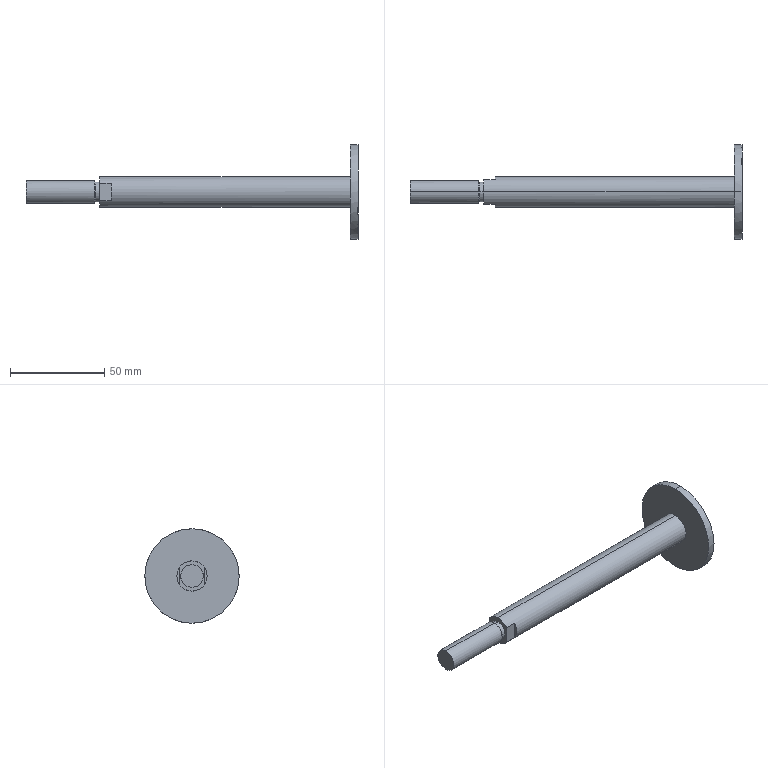Part | SolidWorks | features BaseBody 1, ICE 1 | 1 solid | 18 faces | box 176 x 50 x 50 mm | volume 38817 mm3 | cylinder 8 | plane 8 | cone 2 | commonest cylinder face diameters 10.466 x2 12 x2 16 x2 50 x2
STEP:
#1=CARTESIAN_POINT('',(-46.5,0.,-6.));
#2=VERTEX_POINT('',#1);
#3=CARTESIAN_POINT('',(-46.5,0.,6.));
#4=VERTEX_POINT('',#3);
#5=CARTESIAN_POINT('',(-46.5,0.,0.));
#6=DIRECTION('',(-1.,0.,0.));
#7=DIRECTION('',(0.,0.,1.));
#8=AXIS2_PLACEMENT_3D('',#5,#6,#7);
#9=CIRCLE('',#8,6.);
#10=EDGE_CURVE('',#2,#4,#9,.T.);
#11=ORIENTED_EDGE('',*,*,#10,.F.);
#12=CARTESIAN_POINT('',(-10.355,0.,-6.));
#13=VERTEX_POINT('',#12);
#14=CARTESIAN_POINT('',(-7.5,0.,-6.));
#15=DIRECTION('',(1.,0.,0.));
#16=VECTOR('',#15,1000.);
#17=LINE('',#14,#16);
#18=EDGE_CURVE('',#2,#13,#17,.T.);
#19=ORIENTED_EDGE('',*,*,#18,.T.);
#20=CARTESIAN_POINT('',(-10.355,0.,6.));
#21=VERTEX_POINT('',#20);
#22=CARTESIAN_POINT('',(-10.355,0.,6.));
#23=CARTESIAN_POINT('',(-10.355,-0.7854,6.));
#24=CARTESIAN_POINT('',(-10.355,-1.57,5.844));
#25=CARTESIAN_POINT('',(-10.355,-3.022,5.243));
#26=CARTESIAN_POINT('',(-10.355,-3.687,4.798));
#27=CARTESIAN_POINT('',(-10.355,-4.798,3.687));
#28=CARTESIAN_POINT('',(-10.355,-5.243,3.022));
#29=CARTESIAN_POINT('',(-10.355,-5.844,1.57));
#30=CARTESIAN_POINT('',(-10.355,-6.,0.7854));
#31=CARTESIAN_POINT('',(-10.355,-6.,-0.7854));
#32=CARTESIAN_POINT('',(-10.355,-5.844,-1.57));
#33=CARTESIAN_POINT('',(-10.355,-5.243,-3.022));
#34=CARTESIAN_POINT('',(-10.355,-4.798,-3.687));
#35=CARTESIAN_POINT('',(-10.355,-3.687,-4.798));
#36=CARTESIAN_POINT('',(-10.355,-3.022,-5.243));
#37=CARTESIAN_POINT('',(-10.355,-1.57,-5.844));
#38=CARTESIAN_POINT('',(-10.355,-0.7854,-6.));
#39=CARTESIAN_POINT('',(-10.355,0.,-6.));
#40=B_SPLINE_CURVE_WITH_KNOTS('',3,(#22,#23,#24,#25,#26,#27,#28,#29,#30,#31,#32,#33,#34,#35,#36,#37,#38,#39),.UNSPECIFIED.,.F.,.F.,(4,2,2,2,2,2,2,2,4),(0.,0.125,0.25,0.375,0.5,0.625,0.75,0.875,1.),.UNSPECIFIED.);
#41=EDGE_CURVE('',#21,#13,#40,.T.);
#42=ORIENTED_EDGE('',*,*,#41,.F.);
#43=CARTESIAN_POINT('',(-7.5,0.,6.));
#44=DIRECTION('',(1.,0.,0.));
#45=VECTOR('',#44,1000.);
#46=LINE('',#43,#45);
#47=EDGE_CURVE('',#4,#21,#46,.T.);
#48=ORIENTED_EDGE('',*,*,#47,.F.);
#49=EDGE_LOOP('',(#11,#19,#42,#48));
#50=FACE_OUTER_BOUND('',#49,.T.);
#51=CARTESIAN_POINT('',(-7.5,0.,0.));
#52=DIRECTION('',(1.,0.,0.));
#53=DIRECTION('',(0.,0.,1.));
#54=AXIS2_PLACEMENT_3D('',#51,#52,#53);
#55=CYLINDRICAL_SURFACE('',#54,6.);
#56=ADVANCED_FACE('',(#50),#55,.T.);
#57=CARTESIAN_POINT('',(-7.5,0.,-5.233));
#58=VERTEX_POINT('',#57);
#59=CARTESIAN_POINT('',(-7.5,0.,5.233));
#60=VERTEX_POINT('',#59);
#61=CARTESIAN_POINT('',(-7.5,0.,-5.233));
#62=CARTESIAN_POINT('',(-7.5,0.6937,-5.233));
#63=CARTESIAN_POINT('',(-7.5,1.362,-5.1));
#64=CARTESIAN_POINT('',(-7.5,2.643,-4.569));
#65=CARTESIAN_POINT('',(-7.5,3.21,-4.191));
#66=CARTESIAN_POINT('',(-7.5,4.191,-3.21));
#67=CARTESIAN_POINT('',(-7.5,4.569,-2.643));
#68=CARTESIAN_POINT('',(-7.5,5.1,-1.362));
#69=CARTESIAN_POINT('',(-7.5,5.233,-0.6936));
#70=CARTESIAN_POINT('',(-7.5,5.233,0.6936));
#71=CARTESIAN_POINT('',(-7.5,5.1,1.362));
#72=CARTESIAN_POINT('',(-7.5,4.569,2.643));
#73=CARTESIAN_POINT('',(-7.5,4.191,3.21));
#74=CARTESIAN_POINT('',(-7.5,3.21,4.191));
#75=CARTESIAN_POINT('',(-7.5,2.644,4.569));
#76=CARTESIAN_POINT('',(-7.5,1.362,5.1));
#77=CARTESIAN_POINT('',(-7.5,0.6941,5.233));
#78=CARTESIAN_POINT('',(-7.5,0.,5.233));
#79=B_SPLINE_CURVE_WITH_KNOTS('',3,(#61,#62,#63,#64,#65,#66,#67,#68,#69,#70,#71,#72,#73,#74,#75,#76,#77,#78),.UNSPECIFIED.,.F.,.F.,(4,2,2,2,2,2,2,2,4),(0.,0.125,0.25,0.375,0.5,0.625,0.75,0.875,1.),.UNSPECIFIED.);
#80=EDGE_CURVE('',#58,#60,#79,.T.);
#81=ORIENTED_EDGE('',*,*,#80,.F.);
#82=CARTESIAN_POINT('',(-9.588,0.,-5.233));
#83=VERTEX_POINT('',#82);
#84=CARTESIAN_POINT('',(-9.588,0.,-5.233));
#85=CARTESIAN_POINT('',(-7.5,0.,-5.233));
#86=B_SPLINE_CURVE_WITH_KNOTS('',1,(#84,#85),.UNSPECIFIED.,.F.,.F.,(2,2),(0.,1.),.UNSPECIFIED.);
#87=EDGE_CURVE('',#83,#58,#86,.T.);
#88=ORIENTED_EDGE('',*,*,#87,.F.);
#89=CARTESIAN_POINT('',(-9.588,0.,5.233));
#90=VERTEX_POINT('',#89);
#91=CARTESIAN_POINT('',(-9.588,0.,5.233));
#92=CARTESIAN_POINT('',(-9.588,0.685,5.233));
#93=CARTESIAN_POINT('',(-9.588,1.37,5.097));
#94=CARTESIAN_POINT('',(-9.588,2.635,4.573));
#95=CARTESIAN_POINT('',(-9.588,3.216,4.185));
#96=CARTESIAN_POINT('',(-9.588,4.185,3.216));
#97=CARTESIAN_POINT('',(-9.588,4.573,2.635));
#98=CARTESIAN_POINT('',(-9.588,5.097,1.37));
#99=CARTESIAN_POINT('',(-9.588,5.233,0.685));
#100=CARTESIAN_POINT('',(-9.588,5.233,-0.685));
#101=CARTESIAN_POINT('',(-9.588,5.097,-1.37));
#102=CARTESIAN_POINT('',(-9.588,4.573,-2.635));
#103=CARTESIAN_POINT('',(-9.588,4.185,-3.216));
#104=CARTESIAN_POINT('',(-9.588,3.216,-4.185));
#105=CARTESIAN_POINT('',(-9.588,2.635,-4.573));
#106=CARTESIAN_POINT('',(-9.588,1.37,-5.097));
#107=CARTESIAN_POINT('',(-9.588,0.685,-5.233));
#108=CARTESIAN_POINT('',(-9.588,0.,-5.233));
#109=B_SPLINE_CURVE_WITH_KNOTS('',3,(#91,#92,#93,#94,#95,#96,#97,#98,#99,#100,#101,#102,#103,#104,#105,#106,#107,#108),.UNSPECIFIED.,.F.,.F.,(4,2,2,2,2,2,2,2,4),(0.,0.125,0.25,0.375,0.5,0.625,0.75,0.875,1.),.UNSPECIFIED.);
#110=EDGE_CURVE('',#90,#83,#109,.T.);
#111=ORIENTED_EDGE('',*,*,#110,.F.);
#112=CARTESIAN_POINT('',(-7.5,0.,5.233));
#113=CARTESIAN_POINT('',(-9.588,0.,5.233));
#114=B_SPLINE_CURVE_WITH_KNOTS('',1,(#112,#113),.UNSPECIFIED.,.F.,.F.,(2,2),(0.,1.),.UNSPECIFIED.);
#115=EDGE_CURVE('',#60,#90,#114,.T.);
#116=ORIENTED_EDGE('',*,*,#115,.F.);
#117=EDGE_LOOP('',(#81,#88,#111,#116));
#118=FACE_OUTER_BOUND('',#117,.T.);
#119=CARTESIAN_POINT('',(-7.5,0.,0.));
#120=DIRECTION('',(1.,0.,0.));
#121=DIRECTION('',(0.,0.,-1.));
#122=AXIS2_PLACEMENT_3D('',#119,#120,#121);
#123=CYLINDRICAL_SURFACE('',#122,5.233);
#124=ADVANCED_FACE('',(#118),#123,.T.);
#125=CARTESIAN_POINT('',(-7.5,0.,5.233));
#126=CARTESIAN_POINT('',(-7.5,-0.6937,5.233));
#127=CARTESIAN_POINT('',(-7.5,-1.362,5.1));
#128=CARTESIAN_POINT('',(-7.5,-2.643,4.569));
#129=CARTESIAN_POINT('',(-7.5,-3.21,4.191));
#130=CARTESIAN_POINT('',(-7.5,-4.191,3.21));
#131=CARTESIAN_POINT('',(-7.5,-4.569,2.643));
#132=CARTESIAN_POINT('',(-7.5,-5.1,1.362));
#133=CARTESIAN_POINT('',(-7.5,-5.233,0.6936));
#134=CARTESIAN_POINT('',(-7.5,-5.233,-0.6936));
#135=CARTESIAN_POINT('',(-7.5,-5.1,-1.362));
#136=CARTESIAN_POINT('',(-7.5,-4.569,-2.643));
#137=CARTESIAN_POINT('',(-7.5,-4.191,-3.21));
#138=CARTESIAN_POINT('',(-7.5,-3.21,-4.191));
#139=CARTESIAN_POINT('',(-7.5,-2.644,-4.569));
#140=CARTESIAN_POINT('',(-7.5,-1.362,-5.1));
#141=CARTESIAN_POINT('',(-7.5,-0.6941,-5.233));
#142=CARTESIAN_POINT('',(-7.5,0.,-5.233));
#143=B_SPLINE_CURVE_WITH_KNOTS('',3,(#125,#126,#127,#128,#129,#130,#131,#132,#133,#134,#135,#136,#137,#138,#139,#140,#141,#142),.UNSPECIFIED.,.F.,.F.,(4,2,2,2,2,2,2,2,4),(0.,0.125,0.25,0.375,0.5,0.625,0.75,0.875,1.),.UNSPECIFIED.);
#144=EDGE_CURVE('',#60,#58,#143,.T.);
#145=ORIENTED_EDGE('',*,*,#144,.F.);
#146=ORIENTED_EDGE('',*,*,#115,.T.);
#147=CARTESIAN_POINT('',(-9.588,0.,-5.233));
#148=CARTESIAN_POINT('',(-9.588,-0.685,-5.233));
#149=CARTESIAN_POINT('',(-9.588,-1.37,-5.097));
#150=CARTESIAN_POINT('',(-9.588,-2.635,-4.573));
#151=CARTESIAN_POINT('',(-9.588,-3.216,-4.185));
#152=CARTESIAN_POINT('',(-9.588,-4.185,-3.216));
#153=CARTESIAN_POINT('',(-9.588,-4.573,-2.635));
#154=CARTESIAN_POINT('',(-9.588,-5.097,-1.37));
#155=CARTESIAN_POINT('',(-9.588,-5.233,-0.685));
#156=CARTESIAN_POINT('',(-9.588,-5.233,0.685));
#157=CARTESIAN_POINT('',(-9.588,-5.097,1.37));
#158=CARTESIAN_POINT('',(-9.588,-4.573,2.635));
#159=CARTESIAN_POINT('',(-9.588,-4.185,3.216));
#160=CARTESIAN_POINT('',(-9.588,-3.216,4.185));
#161=CARTESIAN_POINT('',(-9.588,-2.635,4.573));
#162=CARTESIAN_POINT('',(-9.588,-1.37,5.097));
#163=CARTESIAN_POINT('',(-9.588,-0.685,5.233));
#164=CARTESIAN_POINT('',(-9.588,0.,5.233));
#165=B_SPLINE_CURVE_WITH_KNOTS('',3,(#147,#148,#149,#150,#151,#152,#153,#154,#155,#156,#157,#158,#159,#160,#161,#162,#163,#164),.UNSPECIFIED.,.F.,.F.,(4,2,2,2,2,2,2,2,4),(0.,0.125,0.25,0.375,0.5,0.625,0.75,0.875,1.),.UNSPECIFIED.);
#166=EDGE_CURVE('',#83,#90,#165,.T.);
#167=ORIENTED_EDGE('',*,*,#166,.F.);
#168=ORIENTED_EDGE('',*,*,#87,.T.);
#169=EDGE_LOOP('',(#145,#146,#167,#168));
#170=FACE_OUTER_BOUND('',#169,.T.);
#171=CARTESIAN_POINT('',(-7.5,0.,0.));
#172=DIRECTION('',(1.,0.,0.));
#173=DIRECTION('',(0.,0.000000001,1.));
#174=AXIS2_PLACEMENT_3D('',#171,#172,#173);
#175=CYLINDRICAL_SURFACE('',#174,5.233);
#176=ADVANCED_FACE('',(#170),#175,.T.);
#177=ORIENTED_EDGE('',*,*,#18,.F.);
#178=CARTESIAN_POINT('',(-46.5,0.,0.));
#179=DIRECTION('',(-1.,0.,0.));
#180=DIRECTION('',(0.,0.,1.));
#181=AXIS2_PLACEMENT_3D('',#178,#179,#180);
#182=CIRCLE('',#181,6.);
#183=EDGE_CURVE('',#4,#2,#182,.T.);
#184=ORIENTED_EDGE('',*,*,#183,.F.);
#185=ORIENTED_EDGE('',*,*,#47,.T.);
#186=CARTESIAN_POINT('',(-10.355,0.,-6.));
#187=CARTESIAN_POINT('',(-10.355,0.7854,-6.));
#188=CARTESIAN_POINT('',(-10.355,1.57,-5.844));
#189=CARTESIAN_POINT('',(-10.355,3.022,-5.243));
#190=CARTESIAN_POINT('',(-10.355,3.687,-4.798));
#191=CARTESIAN_POINT('',(-10.355,4.798,-3.687));
#192=CARTESIAN_POINT('',(-10.355,5.243,-3.022));
#193=CARTESIAN_POINT('',(-10.355,5.844,-1.57));
#194=CARTESIAN_POINT('',(-10.355,6.,-0.7854));
#195=CARTESIAN_POINT('',(-10.355,6.,0.7854));
#196=CARTESIAN_POINT('',(-10.355,5.844,1.57));
#197=CARTESIAN_POINT('',(-10.355,5.243,3.022));
#198=CARTESIAN_POINT('',(-10.355,4.798,3.687));
#199=CARTESIAN_POINT('',(-10.355,3.687,4.798));
#200=CARTESIAN_POINT('',(-10.355,3.022,5.243));
#201=CARTESIAN_POINT('',(-10.355,1.57,5.844));
#202=CARTESIAN_POINT('',(-10.355,0.7854,6.));
#203=CARTESIAN_POINT('',(-10.355,0.,6.));
#204=B_SPLINE_CURVE_WITH_KNOTS('',3,(#186,#187,#188,#189,#190,#191,#192,#193,#194,#195,#196,#197,#198,#199,#200,#201,#202,#203),.UNSPECIFIED.,.F.,.F.,(4,2,2,2,2,2,2,2,4),(0.,0.125,0.25,0.375,0.5,0.625,0.75,0.875,1.),.UNSPECIFIED.);
#205=EDGE_CURVE('',#13,#21,#204,.T.);
#206=ORIENTED_EDGE('',*,*,#205,.F.);
#207=EDGE_LOOP('',(#177,#184,#185,#206));
#208=FACE_OUTER_BOUND('',#207,.T.);
#209=CARTESIAN_POINT('',(-7.5,0.,0.));
#210=DIRECTION('',(1.,0.,0.));
#211=DIRECTION('',(0.,0.,1.));
#212=AXIS2_PLACEMENT_3D('',#209,#210,#211);
#213=CYLINDRICAL_SURFACE('',#212,6.);
#214=ADVANCED_FACE('',(#208),#213,.T.);
#215=CARTESIAN_POINT('',(129.5,0.,-25.));
#216=VERTEX_POINT('',#215);
#217=CARTESIAN_POINT('',(129.5,0.,25.));
#218=VERTEX_POINT('',#217);
#219=CARTESIAN_POINT('',(129.5,0.,-25.));
#220=CARTESIAN_POINT('',(129.5,1.641,-25.));
#221=CARTESIAN_POINT('',(129.5,3.268,-24.84));
#222=CARTESIAN_POINT('',(129.5,6.487,-24.199));
#223=CARTESIAN_POINT('',(129.5,8.051,-23.725));
#224=CARTESIAN_POINT('',(129.5,11.083,-22.469));
#225=CARTESIAN_POINT('',(129.5,12.525,-21.698));
#226=CARTESIAN_POINT('',(129.5,15.254,-19.875));
#227=CARTESIAN_POINT('',(129.5,16.517,-18.838));
#228=CARTESIAN_POINT('',(129.5,18.838,-16.517));
#229=CARTESIAN_POINT('',(129.5,19.875,-15.254));
#230=CARTESIAN_POINT('',(129.5,21.699,-12.525));
#231=CARTESIAN_POINT('',(129.5,22.469,-11.083));
#232=CARTESIAN_POINT('',(129.5,23.725,-8.051));
#233=CARTESIAN_POINT('',(129.5,24.199,-6.487));
#234=CARTESIAN_POINT('',(129.5,24.84,-3.268));
#235=CARTESIAN_POINT('',(129.5,25.,-1.641));
#236=CARTESIAN_POINT('',(129.5,25.,1.641));
#237=CARTESIAN_POINT('',(129.5,24.84,3.268));
#238=CARTESIAN_POINT('',(129.5,24.199,6.487));
#239=CARTESIAN_POINT('',(129.5,23.725,8.051));
#240=CARTESIAN_POINT('',(129.5,22.469,11.083));
#241=CARTESIAN_POINT('',(129.5,21.698,12.525));
#242=CARTESIAN_POINT('',(129.5,19.875,15.254));
#243=CARTESIAN_POINT('',(129.5,18.838,16.517));
#244=CARTESIAN_POINT('',(129.5,16.517,18.838));
#245=CARTESIAN_POINT('',(129.5,15.254,19.875));
#246=CARTESIAN_POINT('',(129.5,12.525,21.699));
#247=CARTESIAN_POINT('',(129.5,11.083,22.469));
#248=CARTESIAN_POINT('',(129.5,8.051,23.725));
#249=CARTESIAN_POINT('',(129.5,6.487,24.199));
#250=CARTESIAN_POINT('',(129.5,3.267,24.84));
#251=CARTESIAN_POINT('',(129.5,1.642,25.));
#252=CARTESIAN_POINT('',(129.5,0.,25.));
#253=B_SPLINE_CURVE_WITH_KNOTS('',3,(#219,#220,#221,#222,#223,#224,#225,#226,#227,#228,#229,#230,#231,#232,#233,#234,#235,#236,#237,#238,#239,#240,#241,#242,#243,#244,#245,#246,#247,#248,#249,#250,#251,#252),.UNSPECIFIED.,.F.,.F.,(4,2,2,2,2,2,2,2,2,2,2,2,2,2,2,2,4),(0.,0.0625,0.125,0.1875,0.25,0.3125,0.375,0.4375,0.5,0.5625,0.625,0.6875,0.75,0.8125,0.875,0.9375,1.),.UNSPECIFIED.);
#254=EDGE_CURVE('',#216,#218,#253,.T.);
#255=ORIENTED_EDGE('',*,*,#254,.F.);
#256=CARTESIAN_POINT('',(125.5,0.,-25.));
#257=VERTEX_POINT('',#256);
#258=CARTESIAN_POINT('',(125.5,0.,-25.));
#259=CARTESIAN_POINT('',(129.5,0.,-25.));
#260=B_SPLINE_CURVE_WITH_KNOTS('',1,(#258,#259),.UNSPECIFIED.,.F.,.F.,(2,2),(0.,1.),.UNSPECIFIED.);
#261=EDGE_CURVE('',#257,#216,#260,.T.);
#262=ORIENTED_EDGE('',*,*,#261,.F.);
#263=CARTESIAN_POINT('',(125.5,0.,25.));
#264=VERTEX_POINT('',#263);
#265=CARTESIAN_POINT('',(125.5,0.,25.));
#266=CARTESIAN_POINT('',(125.5,1.641,25.));
#267=CARTESIAN_POINT('',(125.5,3.268,24.84));
#268=CARTESIAN_POINT('',(125.5,6.487,24.199));
#269=CARTESIAN_POINT('',(125.5,8.051,23.725));
#270=CARTESIAN_POINT('',(125.5,11.083,22.469));
#271=CARTESIAN_POINT('',(125.5,12.525,21.698));
#272=CARTESIAN_POINT('',(125.5,15.254,19.875));
#273=CARTESIAN_POINT('',(125.5,16.517,18.838));
#274=CARTESIAN_POINT('',(125.5,18.838,16.517));
#275=CARTESIAN_POINT('',(125.5,19.875,15.254));
#276=CARTESIAN_POINT('',(125.5,21.699,12.525));
#277=CARTESIAN_POINT('',(125.5,22.469,11.083));
#278=CARTESIAN_POINT('',(125.5,23.725,8.051));
#279=CARTESIAN_POINT('',(125.5,24.199,6.487));
#280=CARTESIAN_POINT('',(125.5,24.84,3.268));
#281=CARTESIAN_POINT('',(125.5,25.,1.641));
#282=CARTESIAN_POINT('',(125.5,25.,-1.641));
#283=CARTESIAN_POINT('',(125.5,24.84,-3.268));
#284=CARTESIAN_POINT('',(125.5,24.199,-6.487));
#285=CARTESIAN_POINT('',(125.5,23.725,-8.051));
#286=CARTESIAN_POINT('',(125.5,22.469,-11.083));
#287=CARTESIAN_POINT('',(125.5,21.698,-12.525));
#288=CARTESIAN_POINT('',(125.5,19.875,-15.254));
#289=CARTESIAN_POINT('',(125.5,18.838,-16.517));
#290=CARTESIAN_POINT('',(125.5,16.517,-18.838));
#291=CARTESIAN_POINT('',(125.5,15.254,-19.875));
#292=CARTESIAN_POINT('',(125.5,12.525,-21.699));
#293=CARTESIAN_POINT('',(125.5,11.083,-22.469));
#294=CARTESIAN_POINT('',(125.5,8.051,-23.725));
#295=CARTESIAN_POINT('',(125.5,6.487,-24.199));
#296=CARTESIAN_POINT('',(125.5,3.267,-24.84));
#297=CARTESIAN_POINT('',(125.5,1.642,-25.));
#298=CARTESIAN_POINT('',(125.5,0.,-25.));
#299=B_SPLINE_CURVE_WITH_KNOTS('',3,(#265,#266,#267,#268,#269,#270,#271,#272,#273,#274,#275,#276,#277,#278,#279,#280,#281,#282,#283,#284,#285,#286,#287,#288,#289,#290,#291,#292,#293,#294,#295,#296,#297,#298),.UNSPECIFIED.,.F.,.F.,(4,2,2,2,2,2,2,2,2,2,2,2,2,2,2,2,4),(0.,0.0625,0.125,0.1875,0.25,0.3125,0.375,0.4375,0.5,0.5625,0.625,0.6875,0.75,0.8125,0.875,0.9375,1.),.UNSPECIFIED.);
#300=EDGE_CURVE('',#264,#257,#299,.T.);
#301=ORIENTED_EDGE('',*,*,#300,.F.);
#302=CARTESIAN_POINT('',(129.5,0.,25.));
#303=CARTESIAN_POINT('',(125.5,0.,25.));
#304=B_SPLINE_CURVE_WITH_KNOTS('',1,(#302,#303),.UNSPECIFIED.,.F.,.F.,(2,2),(0.,1.),.UNSPECIFIED.);
#305=EDGE_CURVE('',#218,#264,#304,.T.);
#306=ORIENTED_EDGE('',*,*,#305,.F.);
#307=EDGE_LOOP('',(#255,#262,#301,#306));
#308=FACE_OUTER_BOUND('',#307,.T.);
#309=CARTESIAN_POINT('',(129.5,0.,0.));
#310=DIRECTION('',(1.,0.,0.));
#311=DIRECTION('',(0.,0.,-1.));
#312=AXIS2_PLACEMENT_3D('',#309,#310,#311);
#313=CYLINDRICAL_SURFACE('',#312,25.);
#314=ADVANCED_FACE('',(#308),#313,.T.);
#315=CARTESIAN_POINT('',(129.5,0.,25.));
#316=CARTESIAN_POINT('',(129.5,-1.641,25.));
#317=CARTESIAN_POINT('',(129.5,-3.268,24.84));
#318=CARTESIAN_POINT('',(129.5,-6.487,24.199));
#319=CARTESIAN_POINT('',(129.5,-8.051,23.725));
#320=CARTESIAN_POINT('',(129.5,-11.083,22.469));
#321=CARTESIAN_POINT('',(129.5,-12.525,21.698));
#322=CARTESIAN_POINT('',(129.5,-15.254,19.875));
#323=CARTESIAN_POINT('',(129.5,-16.517,18.838));
#324=CARTESIAN_POINT('',(129.5,-18.838,16.517));
#325=CARTESIAN_POINT('',(129.5,-19.875,15.254));
#326=CARTESIAN_POINT('',(129.5,-21.699,12.525));
#327=CARTESIAN_POINT('',(129.5,-22.469,11.083));
#328=CARTESIAN_POINT('',(129.5,-23.725,8.051));
#329=CARTESIAN_POINT('',(129.5,-24.199,6.487));
#330=CARTESIAN_POINT('',(129.5,-24.84,3.268));
#331=CARTESIAN_POINT('',(129.5,-25.,1.641));
#332=CARTESIAN_POINT('',(129.5,-25.,-1.641));
#333=CARTESIAN_POINT('',(129.5,-24.84,-3.268));
#334=CARTESIAN_POINT('',(129.5,-24.199,-6.487));
#335=CARTESIAN_POINT('',(129.5,-23.725,-8.051));
#336=CARTESIAN_POINT('',(129.5,-22.469,-11.083));
#337=CARTESIAN_POINT('',(129.5,-21.698,-12.525));
#338=CARTESIAN_POINT('',(129.5,-19.875,-15.254));
#339=CARTESIAN_POINT('',(129.5,-18.838,-16.517));
#340=CARTESIAN_POINT('',(129.5,-16.517,-18.838));
#341=CARTESIAN_POINT('',(129.5,-15.254,-19.875));
#342=CARTESIAN_POINT('',(129.5,-12.525,-21.699));
#343=CARTESIAN_POINT('',(129.5,-11.083,-22.469));
#344=CARTESIAN_POINT('',(129.5,-8.051,-23.725));
#345=CARTESIAN_POINT('',(129.5,-6.487,-24.199));
#346=CARTESIAN_POINT('',(129.5,-3.267,-24.84));
#347=CARTESIAN_POINT('',(129.5,-1.642,-25.));
#348=CARTESIAN_POINT('',(129.5,0.,-25.));
#349=B_SPLINE_CURVE_WITH_KNOTS('',3,(#315,#316,#317,#318,#319,#320,#321,#322,#323,#324,#325,#326,#327,#328,#329,#330,#331,#332,#333,#334,#335,#336,#337,#338,#339,#340,#341,#342,#343,#344,#345,#346,#347,#348),.UNSPECIFIED.,.F.,.F.,(4,2,2,2,2,2,2,2,2,2,2,2,2,2,2,2,4),(0.,0.0625,0.125,0.1875,0.25,0.3125,0.375,0.4375,0.5,0.5625,0.625,0.6875,0.75,0.8125,0.875,0.9375,1.),.UNSPECIFIED.);
#350=EDGE_CURVE('',#218,#216,#349,.T.);
#351=ORIENTED_EDGE('',*,*,#350,.F.);
#352=ORIENTED_EDGE('',*,*,#305,.T.);
#353=CARTESIAN_POINT('',(125.5,0.,-25.));
#354=CARTESIAN_POINT('',(125.5,-1.641,-25.));
#355=CARTESIAN_POINT('',(125.5,-3.268,-24.84));
#356=CARTESIAN_POINT('',(125.5,-6.487,-24.199));
#357=CARTESIAN_POINT('',(125.5,-8.051,-23.725));
#358=CARTESIAN_POINT('',(125.5,-11.083,-22.469));
#359=CARTESIAN_POINT('',(125.5,-12.525,-21.698));
#360=CARTESIAN_POINT('',(125.5,-15.254,-19.875));
#361=CARTESIAN_POINT('',(125.5,-16.517,-18.838));
#362=CARTESIAN_POINT('',(125.5,-18.838,-16.517));
#363=CARTESIAN_POINT('',(125.5,-19.875,-15.254));
#364=CARTESIAN_POINT('',(125.5,-21.699,-12.525));
#365=CARTESIAN_POINT('',(125.5,-22.469,-11.083));
#366=CARTESIAN_POINT('',(125.5,-23.725,-8.051));
#367=CARTESIAN_POINT('',(125.5,-24.199,-6.487));
#368=CARTESIAN_POINT('',(125.5,-24.84,-3.268));
#369=CARTESIAN_POINT('',(125.5,-25.,-1.641));
#370=CARTESIAN_POINT('',(125.5,-25.,1.641));
#371=CARTESIAN_POINT('',(125.5,-24.84,3.268));
#372=CARTESIAN_POINT('',(125.5,-24.199,6.487));
#373=CARTESIAN_POINT('',(125.5,-23.725,8.051));
#374=CARTESIAN_POINT('',(125.5,-22.469,11.083));
#375=CARTESIAN_POINT('',(125.5,-21.698,12.525));
#376=CARTESIAN_POINT('',(125.5,-19.875,15.254));
#377=CARTESIAN_POINT('',(125.5,-18.838,16.517));
#378=CARTESIAN_POINT('',(125.5,-16.517,18.838));
#379=CARTESIAN_POINT('',(125.5,-15.254,19.875));
#380=CARTESIAN_POINT('',(125.5,-12.525,21.699));
#381=CARTESIAN_POINT('',(125.5,-11.083,22.469));
#382=CARTESIAN_POINT('',(125.5,-8.051,23.725));
#383=CARTESIAN_POINT('',(125.5,-6.487,24.199));
#384=CARTESIAN_POINT('',(125.5,-3.267,24.84));
#385=CARTESIAN_POINT('',(125.5,-1.642,25.));
#386=CARTESIAN_POINT('',(125.5,0.,25.));
#387=B_SPLINE_CURVE_WITH_KNOTS('',3,(#353,#354,#355,#356,#357,#358,#359,#360,#361,#362,#363,#364,#365,#366,#367,#368,#369,#370,#371,#372,#373,#374,#375,#376,#377,#378,#379,#380,#381,#382,#383,#384,#385,#386),.UNSPECIFIED.,.F.,.F.,(4,2,2,2,2,2,2,2,2,2,2,2,2,2,2,2,4),(0.,0.0625,0.125,0.1875,0.25,0.3125,0.375,0.4375,0.5,0.5625,0.625,0.6875,0.75,0.8125,0.875,0.9375,1.),.UNSPECIFIED.);
#388=EDGE_CURVE('',#257,#264,#387,.T.);
#389=ORIENTED_EDGE('',*,*,#388,.F.);
#390=ORIENTED_EDGE('',*,*,#261,.T.);
#391=EDGE_LOOP('',(#351,#352,#389,#390));
#392=FACE_OUTER_BOUND('',#391,.T.);
#393=CARTESIAN_POINT('',(129.5,0.,0.));
#394=DIRECTION('',(1.,0.,0.));
#395=DIRECTION('',(0.,0.,1.));
#396=AXIS2_PLACEMENT_3D('',#393,#394,#395);
#397=CYLINDRICAL_SURFACE('',#396,25.);
#398=ADVANCED_FACE('',(#392),#397,.T.);
#399=CARTESIAN_POINT('',(125.5,0.,-8.));
#400=VERTEX_POINT('',#399);
#401=CARTESIAN_POINT('',(125.5,0.,8.));
#402=VERTEX_POINT('',#401);
#403=CARTESIAN_POINT('',(125.5,0.,-8.));
#404=CARTESIAN_POINT('',(125.5,0.5251,-8.));
#405=CARTESIAN_POINT('',(125.5,1.046,-7.949));
#406=CARTESIAN_POINT('',(125.5,2.076,-7.744));
#407=CARTESIAN_POINT('',(125.5,2.576,-7.592));
#408=CARTESIAN_POINT('',(125.5,3.546,-7.19));
#409=CARTESIAN_POINT('',(125.5,4.008,-6.943));
#410=CARTESIAN_POINT('',(125.5,4.881,-6.36));
#411=CARTESIAN_POINT('',(125.5,5.286,-6.028));
#412=CARTESIAN_POINT('',(125.5,6.028,-5.286));
#413=CARTESIAN_POINT('',(125.5,6.36,-4.881));
#414=CARTESIAN_POINT('',(125.5,6.943,-4.008));
#415=CARTESIAN_POINT('',(125.5,7.19,-3.546));
#416=CARTESIAN_POINT('',(125.5,7.592,-2.577));
#417=CARTESIAN_POINT('',(125.5,7.744,-2.076));
#418=CARTESIAN_POINT('',(125.5,7.949,-1.046));
#419=CARTESIAN_POINT('',(125.5,8.,-0.5249));
#420=CARTESIAN_POINT('',(125.5,8.,0.5249));
#421=CARTESIAN_POINT('',(125.5,7.949,1.046));
#422=CARTESIAN_POINT('',(125.5,7.744,2.076));
#423=CARTESIAN_POINT('',(125.5,7.592,2.576));
#424=CARTESIAN_POINT('',(125.5,7.19,3.546));
#425=CARTESIAN_POINT('',(125.5,6.943,4.008));
#426=CARTESIAN_POINT('',(125.5,6.36,4.881));
#427=CARTESIAN_POINT('',(125.5,6.028,5.286));
#428=CARTESIAN_POINT('',(125.5,5.286,6.028));
#429=CARTESIAN_POINT('',(125.5,4.881,6.36));
#430=CARTESIAN_POINT('',(125.5,4.008,6.943));
#431=CARTESIAN_POINT('',(125.5,3.546,7.19));
#432=CARTESIAN_POINT('',(125.5,2.577,7.592));
#433=CARTESIAN_POINT('',(125.5,2.076,7.744));
#434=CARTESIAN_POINT('',(125.5,1.046,7.949));
#435=CARTESIAN_POINT('',(125.5,0.5255,8.));
#436=CARTESIAN_POINT('',(125.5,0.,8.));
#437=B_SPLINE_CURVE_WITH_KNOTS('',3,(#403,#404,#405,#406,#407,#408,#409,#410,#411,#412,#413,#414,#415,#416,#417,#418,#419,#420,#421,#422,#423,#424,#425,#426,#427,#428,#429,#430,#431,#432,#433,#434,#435,#436),.UNSPECIFIED.,.F.,.F.,(4,2,2,2,2,2,2,2,2,2,2,2,2,2,2,2,4),(0.,0.0625,0.125,0.1875,0.25,0.3125,0.375,0.4375,0.5,0.5625,0.625,0.6875,0.75,0.8125,0.875,0.9375,1.),.UNSPECIFIED.);
#438=EDGE_CURVE('',#400,#402,#437,.T.);
#439=ORIENTED_EDGE('',*,*,#438,.F.);
#440=CARTESIAN_POINT('',(-7.5,0.,-8.));
#441=VERTEX_POINT('',#440);
#442=CARTESIAN_POINT('',(-7.5,0.,-8.));
#443=CARTESIAN_POINT('',(125.5,0.,-8.));
#444=B_SPLINE_CURVE_WITH_KNOTS('',1,(#442,#443),.UNSPECIFIED.,.F.,.F.,(2,2),(0.,1.),.UNSPECIFIED.);
#445=EDGE_CURVE('',#441,#400,#444,.T.);
#446=ORIENTED_EDGE('',*,*,#445,.F.);
#447=CARTESIAN_POINT('',(-7.5,6.5,-4.664));
#448=VERTEX_POINT('',#447);
#449=CARTESIAN_POINT('',(-7.5,6.5,-4.664));
#450=CARTESIAN_POINT('',(-7.5,6.13,-5.18));
#451=CARTESIAN_POINT('',(-7.5,5.703,-5.646));
#452=CARTESIAN_POINT('',(-7.5,4.742,-6.475));
#453=CARTESIAN_POINT('',(-7.5,4.219,-6.827));
#454=CARTESIAN_POINT('',(-7.5,3.088,-7.407));
#455=CARTESIAN_POINT('',(-7.5,2.497,-7.627));
#456=CARTESIAN_POINT('',(-7.5,1.262,-7.925));
#457=CARTESIAN_POINT('',(-7.5,0.6352,-8.));
#458=CARTESIAN_POINT('',(-7.5,0.,-8.));
#459=B_SPLINE_CURVE_WITH_KNOTS('',3,(#449,#450,#451,#452,#453,#454,#455,#456,#457,#458),.UNSPECIFIED.,.F.,.F.,(4,2,2,2,4),(0.,0.25,0.5,0.75,1.),.UNSPECIFIED.);
#460=EDGE_CURVE('',#448,#441,#459,.T.);
#461=ORIENTED_EDGE('',*,*,#460,.F.);
#462=CARTESIAN_POINT('',(-1.3,6.5,-4.664));
#463=VERTEX_POINT('',#462);
#464=CARTESIAN_POINT('',(-1.3,6.5,-4.664));
#465=CARTESIAN_POINT('',(-3.367,6.5,-4.664));
#466=CARTESIAN_POINT('',(-5.433,6.5,-4.664));
#467=CARTESIAN_POINT('',(-7.5,6.5,-4.664));
#468=B_SPLINE_CURVE_WITH_KNOTS('',3,(#464,#465,#466,#467),.UNSPECIFIED.,.F.,.F.,(4,4),(0.,6.2),.UNSPECIFIED.);
#469=EDGE_CURVE('',#463,#448,#468,.T.);
#470=ORIENTED_EDGE('',*,*,#469,.F.);
#471=CARTESIAN_POINT('',(-1.3,6.5,4.664));
#472=VERTEX_POINT('',#471);
#473=CARTESIAN_POINT('',(-1.3,6.5,4.664));
#474=CARTESIAN_POINT('',(-1.3,6.988,3.984));
#475=CARTESIAN_POINT('',(-1.3,7.36,3.246));
#476=CARTESIAN_POINT('',(-1.3,7.872,1.653));
#477=CARTESIAN_POINT('',(-1.3,8.,0.8362));
#478=CARTESIAN_POINT('',(-1.3,8.,-0.8362));
#479=CARTESIAN_POINT('',(-1.3,7.872,-1.653));
#480=CARTESIAN_POINT('',(-1.3,7.36,-3.246));
#481=CARTESIAN_POINT('',(-1.3,6.988,-3.984));
#482=CARTESIAN_POINT('',(-1.3,6.5,-4.664));
#483=B_SPLINE_CURVE_WITH_KNOTS('',3,(#473,#474,#475,#476,#477,#478,#479,#480,#481,#482),.UNSPECIFIED.,.F.,.F.,(4,2,2,2,4),(0.,0.25,0.5,0.75,1.),.UNSPECIFIED.);
#484=EDGE_CURVE('',#472,#463,#483,.T.);
#485=ORIENTED_EDGE('',*,*,#484,.F.);
#486=CARTESIAN_POINT('',(-7.5,6.5,4.664));
#487=VERTEX_POINT('',#486);
#488=CARTESIAN_POINT('',(-7.5,6.5,4.664));
#489=CARTESIAN_POINT('',(-5.433,6.5,4.664));
#490=CARTESIAN_POINT('',(-3.367,6.5,4.664));
#491=CARTESIAN_POINT('',(-1.3,6.5,4.664));
#492=B_SPLINE_CURVE_WITH_KNOTS('',3,(#488,#489,#490,#491),.UNSPECIFIED.,.F.,.F.,(4,4),(0.,6.2),.UNSPECIFIED.);
#493=EDGE_CURVE('',#487,#472,#492,.T.);
#494=ORIENTED_EDGE('',*,*,#493,.F.);
#495=CARTESIAN_POINT('',(-7.5,0.,8.));
#496=VERTEX_POINT('',#495);
#497=CARTESIAN_POINT('',(-7.5,0.,8.));
#498=CARTESIAN_POINT('',(-7.5,0.6349,8.));
#499=CARTESIAN_POINT('',(-7.5,1.263,7.925));
#500=CARTESIAN_POINT('',(-7.5,2.496,7.627));
#501=CARTESIAN_POINT('',(-7.5,3.089,7.407));
#502=CARTESIAN_POINT('',(-7.5,4.218,6.827));
#503=CARTESIAN_POINT('',(-7.5,4.741,6.475));
#504=CARTESIAN_POINT('',(-7.5,5.704,5.645));
#505=CARTESIAN_POINT('',(-7.5,6.13,5.18));
#506=CARTESIAN_POINT('',(-7.5,6.5,4.664));
#507=B_SPLINE_CURVE_WITH_KNOTS('',3,(#497,#498,#499,#500,#501,#502,#503,#504,#505,#506),.UNSPECIFIED.,.F.,.F.,(4,2,2,2,4),(0.,0.25,0.5,0.75,1.),.UNSPECIFIED.);
#508=EDGE_CURVE('',#496,#487,#507,.T.);
#509=ORIENTED_EDGE('',*,*,#508,.F.);
#510=CARTESIAN_POINT('',(125.5,0.,8.));
#511=CARTESIAN_POINT('',(-7.5,0.,8.));
#512=B_SPLINE_CURVE_WITH_KNOTS('',1,(#510,#511),.UNSPECIFIED.,.F.,.F.,(2,2),(0.,1.),.UNSPECIFIED.);
#513=EDGE_CURVE('',#402,#496,#512,.T.);
#514=ORIENTED_EDGE('',*,*,#513,.F.);
#515=EDGE_LOOP('',(#439,#446,#461,#470,#485,#494,#509,#514));
#516=FACE_OUTER_BOUND('',#515,.T.);
#517=CARTESIAN_POINT('',(129.5,0.,0.));
#518=DIRECTION('',(1.,0.,0.));
#519=DIRECTION('',(0.,0.,-1.));
#520=AXIS2_PLACEMENT_3D('',#517,#518,#519);
#521=CYLINDRICAL_SURFACE('',#520,8.);
#522=ADVANCED_FACE('',(#516),#521,.T.);
#523=CARTESIAN_POINT('',(125.5,0.,8.));
#524=CARTESIAN_POINT('',(125.5,-0.5251,8.));
#525=CARTESIAN_POINT('',(125.5,-1.046,7.949));
#526=CARTESIAN_POINT('',(125.5,-2.076,7.744));
#527=CARTESIAN_POINT('',(125.5,-2.576,7.592));
#528=CARTESIAN_POINT('',(125.5,-3.546,7.19));
#529=CARTESIAN_POINT('',(125.5,-4.008,6.943));
#530=CARTESIAN_POINT('',(125.5,-4.881,6.36));
#531=CARTESIAN_POINT('',(125.5,-5.286,6.028));
#532=CARTESIAN_POINT('',(125.5,-6.028,5.286));
#533=CARTESIAN_POINT('',(125.5,-6.36,4.881));
#534=CARTESIAN_POINT('',(125.5,-6.943,4.008));
#535=CARTESIAN_POINT('',(125.5,-7.19,3.546));
#536=CARTESIAN_POINT('',(125.5,-7.592,2.577));
#537=CARTESIAN_POINT('',(125.5,-7.744,2.076));
#538=CARTESIAN_POINT('',(125.5,-7.949,1.046));
#539=CARTESIAN_POINT('',(125.5,-8.,0.5249));
#540=CARTESIAN_POINT('',(125.5,-8.,-0.5249));
#541=CARTESIAN_POINT('',(125.5,-7.949,-1.046));
#542=CARTESIAN_POINT('',(125.5,-7.744,-2.076));
#543=CARTESIAN_POINT('',(125.5,-7.592,-2.576));
#544=CARTESIAN_POINT('',(125.5,-7.19,-3.546));
#545=CARTESIAN_POINT('',(125.5,-6.943,-4.008));
#546=CARTESIAN_POINT('',(125.5,-6.36,-4.881));
#547=CARTESIAN_POINT('',(125.5,-6.028,-5.286));
#548=CARTESIAN_POINT('',(125.5,-5.286,-6.028));
#549=CARTESIAN_POINT('',(125.5,-4.881,-6.36));
#550=CARTESIAN_POINT('',(125.5,-4.008,-6.943));
#551=CARTESIAN_POINT('',(125.5,-3.546,-7.19));
#552=CARTESIAN_POINT('',(125.5,-2.577,-7.592));
#553=CARTESIAN_POINT('',(125.5,-2.076,-7.744));
#554=CARTESIAN_POINT('',(125.5,-1.046,-7.949));
#555=CARTESIAN_POINT('',(125.5,-0.5255,-8.));
#556=CARTESIAN_POINT('',(125.5,0.,-8.));
#557=B_SPLINE_CURVE_WITH_KNOTS('',3,(#523,#524,#525,#526,#527,#528,#529,#530,#531,#532,#533,#534,#535,#536,#537,#538,#539,#540,#541,#542,#543,#544,#545,#546,#547,#548,#549,#550,#551,#552,#553,#554,#555,#556),.UNSPECIFIED.,.F.,.F.,(4,2,2,2,2,2,2,2,2,2,2,2,2,2,2,2,4),(0.,0.0625,0.125,0.1875,0.25,0.3125,0.375,0.4375,0.5,0.5625,0.625,0.6875,0.75,0.8125,0.875,0.9375,1.),.UNSPECIFIED.);
#558=EDGE_CURVE('',#402,#400,#557,.T.);
#559=ORIENTED_EDGE('',*,*,#558,.F.);
#560=ORIENTED_EDGE('',*,*,#513,.T.);
#561=CARTESIAN_POINT('',(-7.5,-6.5,4.664));
#562=VERTEX_POINT('',#561);
#563=CARTESIAN_POINT('',(-7.5,-6.5,4.664));
#564=CARTESIAN_POINT('',(-7.5,-6.13,5.18));
#565=CARTESIAN_POINT('',(-7.5,-5.703,5.646));
#566=CARTESIAN_POINT('',(-7.5,-4.742,6.475));
#567=CARTESIAN_POINT('',(-7.5,-4.219,6.827));
#568=CARTESIAN_POINT('',(-7.5,-3.088,7.407));
#569=CARTESIAN_POINT('',(-7.5,-2.497,7.627));
#570=CARTESIAN_POINT('',(-7.5,-1.262,7.925));
#571=CARTESIAN_POINT('',(-7.5,-0.6352,8.));
#572=CARTESIAN_POINT('',(-7.5,0.,8.));
#573=B_SPLINE_CURVE_WITH_KNOTS('',3,(#563,#564,#565,#566,#567,#568,#569,#570,#571,#572),.UNSPECIFIED.,.F.,.F.,(4,2,2,2,4),(0.,0.25,0.5,0.75,1.),.UNSPECIFIED.);
#574=EDGE_CURVE('',#562,#496,#573,.T.);
#575=ORIENTED_EDGE('',*,*,#574,.F.);
#576=CARTESIAN_POINT('',(-1.3,-6.5,4.664));
#577=VERTEX_POINT('',#576);
#578=CARTESIAN_POINT('',(-1.3,-6.5,4.664));
#579=CARTESIAN_POINT('',(-3.367,-6.5,4.664));
#580=CARTESIAN_POINT('',(-5.433,-6.5,4.664));
#581=CARTESIAN_POINT('',(-7.5,-6.5,4.664));
#582=B_SPLINE_CURVE_WITH_KNOTS('',3,(#578,#579,#580,#581),.UNSPECIFIED.,.F.,.F.,(4,4),(0.,6.2),.UNSPECIFIED.);
#583=EDGE_CURVE('',#577,#562,#582,.T.);
#584=ORIENTED_EDGE('',*,*,#583,.F.);
#585=CARTESIAN_POINT('',(-1.3,-6.5,-4.664));
#586=VERTEX_POINT('',#585);
#587=CARTESIAN_POINT('',(-1.3,-6.5,-4.664));
#588=CARTESIAN_POINT('',(-1.3,-6.988,-3.984));
#589=CARTESIAN_POINT('',(-1.3,-7.36,-3.246));
#590=CARTESIAN_POINT('',(-1.3,-7.872,-1.653));
#591=CARTESIAN_POINT('',(-1.3,-8.,-0.8362));
#592=CARTESIAN_POINT('',(-1.3,-8.,0.8362));
#593=CARTESIAN_POINT('',(-1.3,-7.872,1.653));
#594=CARTESIAN_POINT('',(-1.3,-7.36,3.246));
#595=CARTESIAN_POINT('',(-1.3,-6.988,3.984));
#596=CARTESIAN_POINT('',(-1.3,-6.5,4.664));
#597=B_SPLINE_CURVE_WITH_KNOTS('',3,(#587,#588,#589,#590,#591,#592,#593,#594,#595,#596),.UNSPECIFIED.,.F.,.F.,(4,2,2,2,4),(0.,0.25,0.5,0.75,1.),.UNSPECIFIED.);
#598=EDGE_CURVE('',#586,#577,#597,.T.);
#599=ORIENTED_EDGE('',*,*,#598,.F.);
#600=CARTESIAN_POINT('',(-7.5,-6.5,-4.664));
#601=VERTEX_POINT('',#600);
#602=CARTESIAN_POINT('',(-7.5,-6.5,-4.664));
#603=CARTESIAN_POINT('',(-5.433,-6.5,-4.664));
#604=CARTESIAN_POINT('',(-3.367,-6.5,-4.664));
#605=CARTESIAN_POINT('',(-1.3,-6.5,-4.664));
#606=B_SPLINE_CURVE_WITH_KNOTS('',3,(#602,#603,#604,#605),.UNSPECIFIED.,.F.,.F.,(4,4),(0.,6.2),.UNSPECIFIED.);
#607=EDGE_CURVE('',#601,#586,#606,.T.);
#608=ORIENTED_EDGE('',*,*,#607,.F.);
#609=CARTESIAN_POINT('',(-7.5,0.,-8.));
#610=CARTESIAN_POINT('',(-7.5,-0.6349,-8.));
#611=CARTESIAN_POINT('',(-7.5,-1.263,-7.925));
#612=CARTESIAN_POINT('',(-7.5,-2.496,-7.627));
#613=CARTESIAN_POINT('',(-7.5,-3.089,-7.407));
#614=CARTESIAN_POINT('',(-7.5,-4.218,-6.827));
#615=CARTESIAN_POINT('',(-7.5,-4.741,-6.475));
#616=CARTESIAN_POINT('',(-7.5,-5.704,-5.645));
#617=CARTESIAN_POINT('',(-7.5,-6.13,-5.18));
#618=CARTESIAN_POINT('',(-7.5,-6.5,-4.664));
#619=B_SPLINE_CURVE_WITH_KNOTS('',3,(#609,#610,#611,#612,#613,#614,#615,#616,#617,#618),.UNSPECIFIED.,.F.,.F.,(4,2,2,2,4),(0.,0.25,0.5,0.75,1.),.UNSPECIFIED.);
#620=EDGE_CURVE('',#441,#601,#619,.T.);
#621=ORIENTED_EDGE('',*,*,#620,.F.);
#622=ORIENTED_EDGE('',*,*,#445,.T.);
#623=EDGE_LOOP('',(#559,#560,#575,#584,#599,#608,#621,#622));
#624=FACE_OUTER_BOUND('',#623,.T.);
#625=CARTESIAN_POINT('',(129.5,0.,0.));
#626=DIRECTION('',(1.,0.,0.));
#627=DIRECTION('',(0.,0.,1.));
#628=AXIS2_PLACEMENT_3D('',#625,#626,#627);
#629=CYLINDRICAL_SURFACE('',#628,8.);
#630=ADVANCED_FACE('',(#624),#629,.T.);
#631=ORIENTED_EDGE('',*,*,#205,.T.);
#632=CARTESIAN_POINT('',(-9.588,0.,5.233));
#633=CARTESIAN_POINT('',(-10.355,0.,6.));
#634=B_SPLINE_CURVE_WITH_KNOTS('',1,(#632,#633),.UNSPECIFIED.,.F.,.F.,(2,2),(0.,1.),.UNSPECIFIED.);
#635=EDGE_CURVE('',#90,#21,#634,.T.);
#636=ORIENTED_EDGE('',*,*,#635,.F.);
#637=ORIENTED_EDGE('',*,*,#110,.T.);
#638=CARTESIAN_POINT('',(-10.355,0.,-6.));
#639=CARTESIAN_POINT('',(-9.588,0.,-5.233));
#640=B_SPLINE_CURVE_WITH_KNOTS('',1,(#638,#639),.UNSPECIFIED.,.F.,.F.,(2,2),(0.,1.),.UNSPECIFIED.);
#641=EDGE_CURVE('',#13,#83,#640,.T.);
#642=ORIENTED_EDGE('',*,*,#641,.F.);
#643=EDGE_LOOP('',(#631,#636,#637,#642));
#644=FACE_OUTER_BOUND('',#643,.T.);
#645=CARTESIAN_POINT('',(-10.355,0.,0.));
#646=DIRECTION('',(-1.,0.,0.));
#647=DIRECTION('',(0.,0.,1.));
#648=AXIS2_PLACEMENT_3D('',#645,#646,#647);
#649=CONICAL_SURFACE('',#648,6.,0.7854);
#650=ADVANCED_FACE('',(#644),#649,.T.);
#651=ORIENTED_EDGE('',*,*,#166,.T.);
#652=ORIENTED_EDGE('',*,*,#635,.T.);
#653=ORIENTED_EDGE('',*,*,#41,.T.);
#654=ORIENTED_EDGE('',*,*,#641,.T.);
#655=EDGE_LOOP('',(#651,#652,#653,#654));
#656=FACE_OUTER_BOUND('',#655,.T.);
#657=CARTESIAN_POINT('',(-10.355,0.,0.));
#658=DIRECTION('',(-1.,0.,0.));
#659=DIRECTION('',(0.,0.,-1.));
#660=AXIS2_PLACEMENT_3D('',#657,#658,#659);
#661=CONICAL_SURFACE('',#660,6.,0.7854);
#662=ADVANCED_FACE('',(#656),#661,.T.);
#663=CARTESIAN_POINT('',(-1.3,6.5,4.664));
#664=CARTESIAN_POINT('',(-1.3,6.5,1.555));
#665=CARTESIAN_POINT('',(-1.3,6.5,-1.555));
#666=CARTESIAN_POINT('',(-1.3,6.5,-4.664));
#667=B_SPLINE_CURVE_WITH_KNOTS('',3,(#663,#664,#665,#666),.UNSPECIFIED.,.F.,.F.,(4,4),(0.,9.327),.UNSPECIFIED.);
#668=EDGE_CURVE('',#472,#463,#667,.T.);
#669=ORIENTED_EDGE('',*,*,#668,.F.);
#670=ORIENTED_EDGE('',*,*,#484,.T.);
#671=EDGE_LOOP('',(#669,#670));
#672=FACE_OUTER_BOUND('',#671,.T.);
#673=CARTESIAN_POINT('',(-1.3,0.,0.));
#674=DIRECTION('',(1.,0.,0.));
#675=DIRECTION('',(0.,1.,0.));
#676=AXIS2_PLACEMENT_3D('',#673,#674,#675);
#677=PLANE('',#676);
#678=ADVANCED_FACE('',(#672),#677,.F.);
#679=ORIENTED_EDGE('',*,*,#469,.T.);
#680=CARTESIAN_POINT('',(-7.5,6.5,4.664));
#681=CARTESIAN_POINT('',(-7.5,6.5,1.555));
#682=CARTESIAN_POINT('',(-7.5,6.5,-1.555));
#683=CARTESIAN_POINT('',(-7.5,6.5,-4.664));
#684=B_SPLINE_CURVE_WITH_KNOTS('',3,(#680,#681,#682,#683),.UNSPECIFIED.,.F.,.F.,(4,4),(0.,9.327),.UNSPECIFIED.);
#685=EDGE_CURVE('',#487,#448,#684,.T.);
#686=ORIENTED_EDGE('',*,*,#685,.F.);
#687=ORIENTED_EDGE('',*,*,#493,.T.);
#688=ORIENTED_EDGE('',*,*,#668,.T.);
#689=EDGE_LOOP('',(#679,#686,#687,#688));
#690=FACE_OUTER_BOUND('',#689,.T.);
#691=CARTESIAN_POINT('',(-1.3,6.5,-13.));
#692=DIRECTION('',(0.,-1.,0.));
#693=DIRECTION('',(0.,0.,-1.));
#694=AXIS2_PLACEMENT_3D('',#691,#692,#693);
#695=PLANE('',#694);
#696=ADVANCED_FACE('',(#690),#695,.F.);
#697=CARTESIAN_POINT('',(-7.5,-6.5,-4.664));
#698=CARTESIAN_POINT('',(-7.5,-6.5,-1.555));
#699=CARTESIAN_POINT('',(-7.5,-6.5,1.555));
#700=CARTESIAN_POINT('',(-7.5,-6.5,4.664));
#701=B_SPLINE_CURVE_WITH_KNOTS('',3,(#697,#698,#699,#700),.UNSPECIFIED.,.F.,.F.,(4,4),(0.,9.327),.UNSPECIFIED.);
#702=EDGE_CURVE('',#601,#562,#701,.T.);
#703=ORIENTED_EDGE('',*,*,#702,.F.);
#704=ORIENTED_EDGE('',*,*,#607,.T.);
#705=CARTESIAN_POINT('',(-1.3,-6.5,4.664));
#706=CARTESIAN_POINT('',(-1.3,-6.5,1.555));
#707=CARTESIAN_POINT('',(-1.3,-6.5,-1.555));
#708=CARTESIAN_POINT('',(-1.3,-6.5,-4.664));
#709=B_SPLINE_CURVE_WITH_KNOTS('',3,(#705,#706,#707,#708),.UNSPECIFIED.,.F.,.F.,(4,4),(0.,9.327),.UNSPECIFIED.);
#710=EDGE_CURVE('',#577,#586,#709,.T.);
#711=ORIENTED_EDGE('',*,*,#710,.F.);
#712=ORIENTED_EDGE('',*,*,#583,.T.);
#713=EDGE_LOOP('',(#703,#704,#711,#712));
#714=FACE_OUTER_BOUND('',#713,.T.);
#715=CARTESIAN_POINT('',(-1.3,-6.5,13.));
#716=DIRECTION('',(0.,1.,0.));
#717=DIRECTION('',(1.,0.,0.));
#718=AXIS2_PLACEMENT_3D('',#715,#716,#717);
#719=PLANE('',#718);
#720=ADVANCED_FACE('',(#714),#719,.F.);
#721=ORIENTED_EDGE('',*,*,#710,.T.);
#722=ORIENTED_EDGE('',*,*,#598,.T.);
#723=EDGE_LOOP('',(#721,#722));
#724=FACE_OUTER_BOUND('',#723,.T.);
#725=CARTESIAN_POINT('',(-1.3,0.,0.));
#726=DIRECTION('',(1.,0.,0.));
#727=DIRECTION('',(0.,1.,0.));
#728=AXIS2_PLACEMENT_3D('',#725,#726,#727);
#729=PLANE('',#728);
#730=ADVANCED_FACE('',(#724),#729,.F.);
#731=ORIENTED_EDGE('',*,*,#350,.T.);
#732=ORIENTED_EDGE('',*,*,#254,.T.);
#733=EDGE_LOOP('',(#731,#732));
#734=FACE_OUTER_BOUND('',#733,.T.);
#735=CARTESIAN_POINT('',(129.5,25.,0.));
#736=DIRECTION('',(-1.,0.,0.));
#737=DIRECTION('',(0.,0.,1.));
#738=AXIS2_PLACEMENT_3D('',#735,#736,#737);
#739=PLANE('',#738);
#740=ADVANCED_FACE('',(#734),#739,.F.);
#741=ORIENTED_EDGE('',*,*,#558,.T.);
#742=ORIENTED_EDGE('',*,*,#438,.T.);
#743=EDGE_LOOP('',(#741,#742));
#744=FACE_BOUND('',#743,.T.);
#745=ORIENTED_EDGE('',*,*,#300,.T.);
#746=ORIENTED_EDGE('',*,*,#388,.T.);
#747=EDGE_LOOP('',(#745,#746));
#748=FACE_OUTER_BOUND('',#747,.T.);
#749=CARTESIAN_POINT('',(125.5,8.,0.));
#750=DIRECTION('',(1.,0.,0.));
#751=DIRECTION('',(0.,1.,0.));
#752=AXIS2_PLACEMENT_3D('',#749,#750,#751);
#753=PLANE('',#752);
#754=ADVANCED_FACE('',(#744,#748),#753,.F.);
#755=ORIENTED_EDGE('',*,*,#144,.T.);
#756=ORIENTED_EDGE('',*,*,#80,.T.);
#757=EDGE_LOOP('',(#755,#756));
#758=FACE_BOUND('',#757,.T.);
#759=ORIENTED_EDGE('',*,*,#685,.T.);
#760=ORIENTED_EDGE('',*,*,#460,.T.);
#761=ORIENTED_EDGE('',*,*,#620,.T.);
#762=ORIENTED_EDGE('',*,*,#702,.T.);
#763=ORIENTED_EDGE('',*,*,#574,.T.);
#764=ORIENTED_EDGE('',*,*,#508,.T.);
#765=EDGE_LOOP('',(#759,#760,#761,#762,#763,#764));
#766=FACE_OUTER_BOUND('',#765,.T.);
#767=CARTESIAN_POINT('',(-7.5,0.,0.));
#768=DIRECTION('',(1.,0.,0.));
#769=DIRECTION('',(0.,1.,0.));
#770=AXIS2_PLACEMENT_3D('',#767,#768,#769);
#771=PLANE('',#770);
#772=ADVANCED_FACE('',(#758,#766),#771,.F.);
#773=ORIENTED_EDGE('',*,*,#183,.T.);
#774=ORIENTED_EDGE('',*,*,#10,.T.);
#775=EDGE_LOOP('',(#773,#774));
#776=FACE_OUTER_BOUND('',#775,.T.);
#777=CARTESIAN_POINT('',(-46.5,0.,0.));
#778=DIRECTION('',(-1.,0.,0.));
#779=DIRECTION('',(0.,0.,1.));
#780=AXIS2_PLACEMENT_3D('',#777,#778,#779);
#781=PLANE('',#780);
#782=ADVANCED_FACE('',(#776),#781,.T.);
#783=CLOSED_SHELL('',(#56,#124,#176,#214,#314,#398,#522,#630,#650,#662,#678,#696,#720,#730,#740,#754,#772,#782));
#784=MANIFOLD_SOLID_BREP('',#783);
#785=CARTESIAN_POINT('',(0.,0.,0.));
#786=DIRECTION('',(0.,0.,1.));
#787=DIRECTION('',(1.,0.,0.));
#788=AXIS2_PLACEMENT_3D('',#785,#786,#787);
#789=(LENGTH_UNIT()NAMED_UNIT(*)SI_UNIT(.MILLI.,.METRE.));
#790=UNCERTAINTY_MEASURE_WITH_UNIT(LENGTH_MEASURE(0.00001),#789,'','');
#791=(NAMED_UNIT(*)PLANE_ANGLE_UNIT()SI_UNIT($,.RADIAN.));
#792=(NAMED_UNIT(*)SI_UNIT($,.STERADIAN.)SOLID_ANGLE_UNIT());
#793=(GEOMETRIC_REPRESENTATION_CONTEXT(3)GLOBAL_UNCERTAINTY_ASSIGNED_CONTEXT((#790))GLOBAL_UNIT_ASSIGNED_CONTEXT((#789,#791,#792))REPRESENTATION_CONTEXT('',''));
#794=ADVANCED_BREP_SHAPE_REPRESENTATION('',(#784,#788),#793);